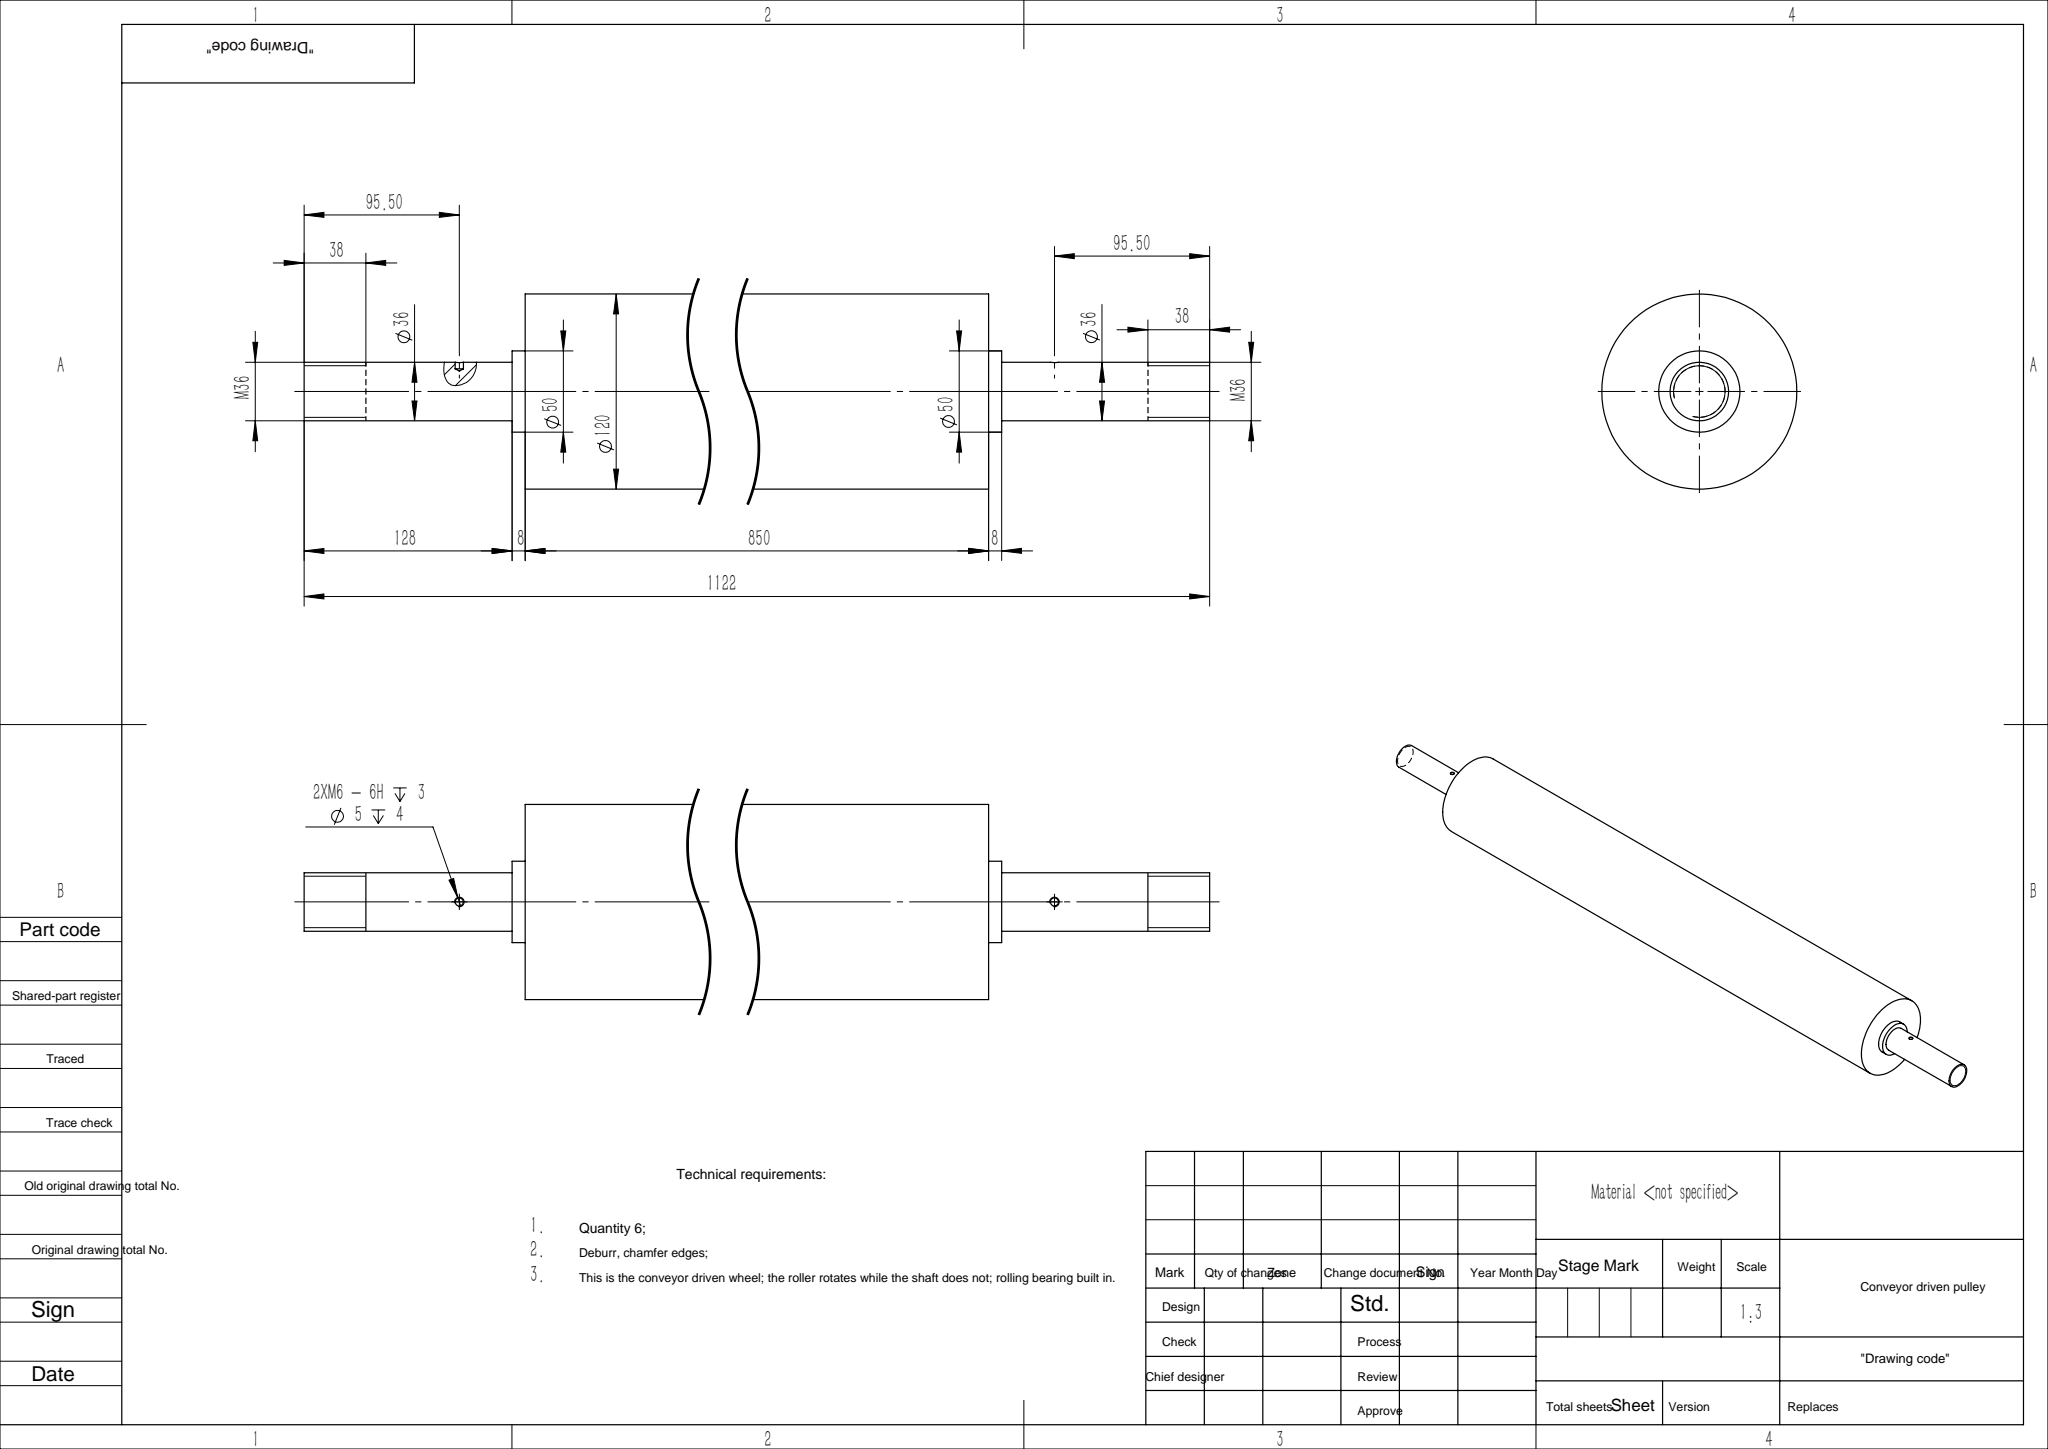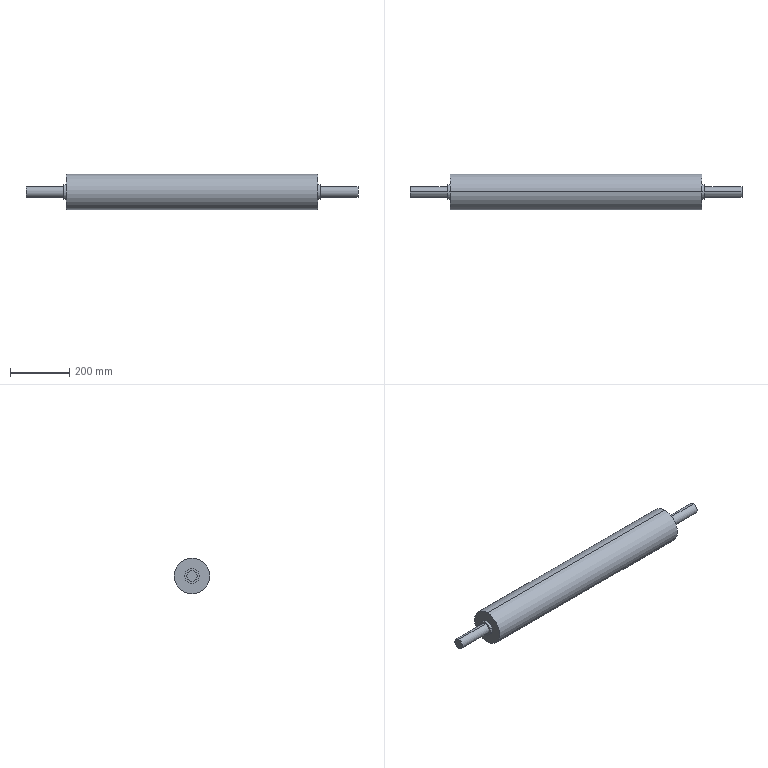Part | SolidWorks | features 3DProfileFeature 1, HoleWzd 1, MirrorPattern 1, Revolution 1 | 1 solid | 24 faces | box 1122 x 120 x 120 mm | volume 9905091 mm3 | cylinder 14 | plane 6 | cone 4 | commonest cylinder face diameters 5 x4 36 x4 50 x4 120 x2
STEP:
#1=CARTESIAN_POINT('',(-465.5,12.557,0.));
#2=VERTEX_POINT('',#1);
#3=CARTESIAN_POINT('',(-465.5,14.,2.5));
#4=VERTEX_POINT('',#3);
#5=CARTESIAN_POINT('',(-465.5,14.,2.5));
#6=DIRECTION('',(0.,0.5,0.866));
#7=VECTOR('',#6,1000.);
#8=LINE('',#5,#7);
#9=EDGE_CURVE('',#2,#4,#8,.T.);
#10=ORIENTED_EDGE('',*,*,#9,.F.);
#11=CARTESIAN_POINT('',(-465.5,14.,-2.5));
#12=VERTEX_POINT('',#11);
#13=CARTESIAN_POINT('',(-465.5,14.,-2.5));
#14=DIRECTION('',(0.,0.5,-0.866));
#15=VECTOR('',#14,1000.);
#16=LINE('',#13,#15);
#17=EDGE_CURVE('',#2,#12,#16,.T.);
#18=ORIENTED_EDGE('',*,*,#17,.T.);
#19=CARTESIAN_POINT('',(-465.5,14.,0.));
#20=DIRECTION('',(0.,1.,0.));
#21=DIRECTION('',(0.,0.,1.));
#22=AXIS2_PLACEMENT_3D('',#19,#20,#21);
#23=CIRCLE('',#22,2.5);
#24=EDGE_CURVE('',#12,#4,#23,.T.);
#25=ORIENTED_EDGE('',*,*,#24,.T.);
#26=EDGE_LOOP('',(#10,#18,#25));
#27=FACE_OUTER_BOUND('',#26,.T.);
#28=CARTESIAN_POINT('',(-465.5,14.,0.));
#29=DIRECTION('',(0.,1.,0.));
#30=DIRECTION('',(0.,0.,1.));
#31=AXIS2_PLACEMENT_3D('',#28,#29,#30);
#32=CONICAL_SURFACE('',#31,2.5,1.047);
#33=ADVANCED_FACE('',(#27),#32,.F.);
#34=ORIENTED_EDGE('',*,*,#24,.F.);
#35=CARTESIAN_POINT('',(-465.5,17.826,-2.5));
#36=VERTEX_POINT('',#35);
#37=CARTESIAN_POINT('',(-465.5,18.,-2.5));
#38=DIRECTION('',(0.,1.,0.));
#39=VECTOR('',#38,1000.);
#40=LINE('',#37,#39);
#41=EDGE_CURVE('',#12,#36,#40,.T.);
#42=ORIENTED_EDGE('',*,*,#41,.T.);
#43=CARTESIAN_POINT('',(-465.5,17.826,2.5));
#44=VERTEX_POINT('',#43);
#45=CARTESIAN_POINT('',(-465.5,17.826,2.5));
#46=CARTESIAN_POINT('',(-465.665,17.826,2.5));
#47=CARTESIAN_POINT('',(-465.828,17.828,2.484));
#48=CARTESIAN_POINT('',(-466.148,17.837,2.42));
#49=CARTESIAN_POINT('',(-466.307,17.843,2.372));
#50=CARTESIAN_POINT('',(-466.609,17.859,2.246));
#51=CARTESIAN_POINT('',(-466.753,17.869,2.17));
#52=CARTESIAN_POINT('',(-467.025,17.89,1.988));
#53=CARTESIAN_POINT('',(-467.153,17.902,1.883));
#54=CARTESIAN_POINT('',(-467.383,17.924,1.652));
#55=CARTESIAN_POINT('',(-467.487,17.936,1.526));
#56=CARTESIAN_POINT('',(-467.669,17.957,1.253));
#57=CARTESIAN_POINT('',(-467.747,17.966,1.108));
#58=CARTESIAN_POINT('',(-467.872,17.983,0.8072));
#59=CARTESIAN_POINT('',(-467.92,17.989,0.6494));
#60=CARTESIAN_POINT('',(-467.984,17.998,0.3266));
#61=CARTESIAN_POINT('',(-468.,18.,0.1642));
#62=CARTESIAN_POINT('',(-468.,18.,-0.1624));
#63=CARTESIAN_POINT('',(-467.984,17.998,-0.3282));
#64=CARTESIAN_POINT('',(-467.92,17.989,-0.649));
#65=CARTESIAN_POINT('',(-467.873,17.983,-0.805));
#66=CARTESIAN_POINT('',(-467.747,17.967,-1.108));
#67=CARTESIAN_POINT('',(-467.669,17.957,-1.254));
#68=CARTESIAN_POINT('',(-467.488,17.936,-1.525));
#69=CARTESIAN_POINT('',(-467.384,17.924,-1.651));
#70=CARTESIAN_POINT('',(-467.151,17.901,-1.884));
#71=CARTESIAN_POINT('',(-467.025,17.89,-1.987));
#72=CARTESIAN_POINT('',(-466.755,17.869,-2.168));
#73=CARTESIAN_POINT('',(-466.608,17.859,-2.247));
#74=CARTESIAN_POINT('',(-466.306,17.843,-2.372));
#75=CARTESIAN_POINT('',(-466.15,17.837,-2.42));
#76=CARTESIAN_POINT('',(-465.829,17.828,-2.484));
#77=CARTESIAN_POINT('',(-465.663,17.826,-2.5));
#78=CARTESIAN_POINT('',(-465.5,17.826,-2.5));
#79=B_SPLINE_CURVE_WITH_KNOTS('',3,(#45,#46,#47,#48,#49,#50,#51,#52,#53,#54,#55,#56,#57,#58,#59,#60,#61,#62,#63,#64,#65,#66,#67,#68,#69,#70,#71,#72,#73,#74,#75,#76,#77,#78),.UNSPECIFIED.,.F.,.F.,(4,2,2,2,2,2,2,2,2,2,2,2,2,2,2,2,4),(0.,0.0004891,0.0009782,0.001467,0.001956,0.002445,0.002935,0.003424,0.003913,0.004402,0.004891,0.00538,0.005869,0.006358,0.006847,0.007336,0.007826),.UNSPECIFIED.);
#80=EDGE_CURVE('',#44,#36,#79,.T.);
#81=ORIENTED_EDGE('',*,*,#80,.F.);
#82=CARTESIAN_POINT('',(-465.5,18.,2.5));
#83=DIRECTION('',(0.,1.,0.));
#84=VECTOR('',#83,1000.);
#85=LINE('',#82,#84);
#86=EDGE_CURVE('',#4,#44,#85,.T.);
#87=ORIENTED_EDGE('',*,*,#86,.F.);
#88=EDGE_LOOP('',(#34,#42,#81,#87));
#89=FACE_OUTER_BOUND('',#88,.T.);
#90=CARTESIAN_POINT('',(-465.5,18.,0.));
#91=DIRECTION('',(0.,1.,0.));
#92=DIRECTION('',(0.,0.,1.));
#93=AXIS2_PLACEMENT_3D('',#90,#91,#92);
#94=CYLINDRICAL_SURFACE('',#93,2.5);
#95=ADVANCED_FACE('',(#89),#94,.F.);
#96=CARTESIAN_POINT('',(465.5,12.557,0.));
#97=VERTEX_POINT('',#96);
#98=CARTESIAN_POINT('',(465.5,14.,2.5));
#99=VERTEX_POINT('',#98);
#100=CARTESIAN_POINT('',(465.5,14.,2.5));
#101=DIRECTION('',(0.,0.5,0.866));
#102=VECTOR('',#101,1000.);
#103=LINE('',#100,#102);
#104=EDGE_CURVE('',#97,#99,#103,.T.);
#105=ORIENTED_EDGE('',*,*,#104,.F.);
#106=CARTESIAN_POINT('',(465.5,14.,-2.5));
#107=VERTEX_POINT('',#106);
#108=CARTESIAN_POINT('',(465.5,14.,-2.5));
#109=DIRECTION('',(0.,0.5,-0.866));
#110=VECTOR('',#109,1000.);
#111=LINE('',#108,#110);
#112=EDGE_CURVE('',#97,#107,#111,.T.);
#113=ORIENTED_EDGE('',*,*,#112,.T.);
#114=CARTESIAN_POINT('',(465.5,14.,0.));
#115=DIRECTION('',(0.,1.,0.));
#116=DIRECTION('',(0.,0.,1.));
#117=AXIS2_PLACEMENT_3D('',#114,#115,#116);
#118=CIRCLE('',#117,2.5);
#119=EDGE_CURVE('',#107,#99,#118,.T.);
#120=ORIENTED_EDGE('',*,*,#119,.T.);
#121=EDGE_LOOP('',(#105,#113,#120));
#122=FACE_OUTER_BOUND('',#121,.T.);
#123=CARTESIAN_POINT('',(465.5,14.,0.));
#124=DIRECTION('',(0.,1.,0.));
#125=DIRECTION('',(0.,0.,1.));
#126=AXIS2_PLACEMENT_3D('',#123,#124,#125);
#127=CONICAL_SURFACE('',#126,2.5,1.047);
#128=ADVANCED_FACE('',(#122),#127,.F.);
#129=ORIENTED_EDGE('',*,*,#119,.F.);
#130=CARTESIAN_POINT('',(465.5,17.826,-2.5));
#131=VERTEX_POINT('',#130);
#132=CARTESIAN_POINT('',(465.5,18.,-2.5));
#133=DIRECTION('',(0.,1.,0.));
#134=VECTOR('',#133,1000.);
#135=LINE('',#132,#134);
#136=EDGE_CURVE('',#107,#131,#135,.T.);
#137=ORIENTED_EDGE('',*,*,#136,.T.);
#138=CARTESIAN_POINT('',(465.5,17.826,2.5));
#139=VERTEX_POINT('',#138);
#140=CARTESIAN_POINT('',(465.5,17.826,2.5));
#141=CARTESIAN_POINT('',(465.335,17.826,2.5));
#142=CARTESIAN_POINT('',(465.172,17.828,2.484));
#143=CARTESIAN_POINT('',(464.852,17.837,2.42));
#144=CARTESIAN_POINT('',(464.693,17.843,2.372));
#145=CARTESIAN_POINT('',(464.391,17.859,2.246));
#146=CARTESIAN_POINT('',(464.247,17.869,2.17));
#147=CARTESIAN_POINT('',(463.975,17.89,1.988));
#148=CARTESIAN_POINT('',(463.847,17.902,1.883));
#149=CARTESIAN_POINT('',(463.617,17.924,1.652));
#150=CARTESIAN_POINT('',(463.513,17.936,1.526));
#151=CARTESIAN_POINT('',(463.331,17.957,1.253));
#152=CARTESIAN_POINT('',(463.253,17.966,1.108));
#153=CARTESIAN_POINT('',(463.128,17.983,0.8072));
#154=CARTESIAN_POINT('',(463.08,17.989,0.6494));
#155=CARTESIAN_POINT('',(463.016,17.998,0.3266));
#156=CARTESIAN_POINT('',(463.,18.,0.1642));
#157=CARTESIAN_POINT('',(463.,18.,-0.1624));
#158=CARTESIAN_POINT('',(463.016,17.998,-0.3282));
#159=CARTESIAN_POINT('',(463.08,17.989,-0.649));
#160=CARTESIAN_POINT('',(463.127,17.983,-0.805));
#161=CARTESIAN_POINT('',(463.253,17.967,-1.108));
#162=CARTESIAN_POINT('',(463.331,17.957,-1.254));
#163=CARTESIAN_POINT('',(463.512,17.936,-1.525));
#164=CARTESIAN_POINT('',(463.616,17.924,-1.651));
#165=CARTESIAN_POINT('',(463.849,17.901,-1.884));
#166=CARTESIAN_POINT('',(463.975,17.89,-1.987));
#167=CARTESIAN_POINT('',(464.245,17.869,-2.168));
#168=CARTESIAN_POINT('',(464.392,17.859,-2.247));
#169=CARTESIAN_POINT('',(464.694,17.843,-2.372));
#170=CARTESIAN_POINT('',(464.85,17.837,-2.42));
#171=CARTESIAN_POINT('',(465.171,17.828,-2.484));
#172=CARTESIAN_POINT('',(465.337,17.826,-2.5));
#173=CARTESIAN_POINT('',(465.5,17.826,-2.5));
#174=B_SPLINE_CURVE_WITH_KNOTS('',3,(#140,#141,#142,#143,#144,#145,#146,#147,#148,#149,#150,#151,#152,#153,#154,#155,#156,#157,#158,#159,#160,#161,#162,#163,#164,#165,#166,#167,#168,#169,#170,#171,#172,#173),.UNSPECIFIED.,.F.,.F.,(4,2,2,2,2,2,2,2,2,2,2,2,2,2,2,2,4),(0.,0.0004891,0.0009782,0.001467,0.001956,0.002445,0.002935,0.003424,0.003913,0.004402,0.004891,0.00538,0.005869,0.006358,0.006847,0.007336,0.007826),.UNSPECIFIED.);
#175=EDGE_CURVE('',#139,#131,#174,.T.);
#176=ORIENTED_EDGE('',*,*,#175,.F.);
#177=CARTESIAN_POINT('',(465.5,18.,2.5));
#178=DIRECTION('',(0.,1.,0.));
#179=VECTOR('',#178,1000.);
#180=LINE('',#177,#179);
#181=EDGE_CURVE('',#99,#139,#180,.T.);
#182=ORIENTED_EDGE('',*,*,#181,.F.);
#183=EDGE_LOOP('',(#129,#137,#176,#182));
#184=FACE_OUTER_BOUND('',#183,.T.);
#185=CARTESIAN_POINT('',(465.5,18.,0.));
#186=DIRECTION('',(0.,1.,0.));
#187=DIRECTION('',(0.,0.,1.));
#188=AXIS2_PLACEMENT_3D('',#185,#186,#187);
#189=CYLINDRICAL_SURFACE('',#188,2.5);
#190=ADVANCED_FACE('',(#184),#189,.F.);
#191=CARTESIAN_POINT('',(425.,0.,60.));
#192=VERTEX_POINT('',#191);
#193=CARTESIAN_POINT('',(425.,0.,-60.));
#194=VERTEX_POINT('',#193);
#195=CARTESIAN_POINT('',(425.,0.,0.));
#196=DIRECTION('',(-1.,0.,0.));
#197=DIRECTION('',(0.,0.,1.));
#198=AXIS2_PLACEMENT_3D('',#195,#196,#197);
#199=CIRCLE('',#198,60.);
#200=EDGE_CURVE('',#192,#194,#199,.T.);
#201=ORIENTED_EDGE('',*,*,#200,.T.);
#202=CARTESIAN_POINT('',(-425.,0.,-60.));
#203=VERTEX_POINT('',#202);
#204=CARTESIAN_POINT('',(0.,0.,-60.));
#205=DIRECTION('',(-1.,0.,0.));
#206=VECTOR('',#205,1000.);
#207=LINE('',#204,#206);
#208=EDGE_CURVE('',#194,#203,#207,.T.);
#209=ORIENTED_EDGE('',*,*,#208,.T.);
#210=CARTESIAN_POINT('',(-425.,0.,60.));
#211=VERTEX_POINT('',#210);
#212=CARTESIAN_POINT('',(-425.,0.,0.));
#213=DIRECTION('',(-1.,0.,0.));
#214=DIRECTION('',(0.,0.,1.));
#215=AXIS2_PLACEMENT_3D('',#212,#213,#214);
#216=CIRCLE('',#215,60.);
#217=EDGE_CURVE('',#211,#203,#216,.T.);
#218=ORIENTED_EDGE('',*,*,#217,.F.);
#219=CARTESIAN_POINT('',(0.,0.,60.));
#220=DIRECTION('',(-1.,0.,0.));
#221=VECTOR('',#220,1000.);
#222=LINE('',#219,#221);
#223=EDGE_CURVE('',#192,#211,#222,.T.);
#224=ORIENTED_EDGE('',*,*,#223,.F.);
#225=EDGE_LOOP('',(#201,#209,#218,#224));
#226=FACE_OUTER_BOUND('',#225,.T.);
#227=CARTESIAN_POINT('',(0.,0.,0.));
#228=DIRECTION('',(-1.,0.,0.));
#229=DIRECTION('',(0.,0.,1.));
#230=AXIS2_PLACEMENT_3D('',#227,#228,#229);
#231=CYLINDRICAL_SURFACE('',#230,60.);
#232=ADVANCED_FACE('',(#226),#231,.T.);
#233=CARTESIAN_POINT('',(-425.,0.,25.));
#234=VERTEX_POINT('',#233);
#235=CARTESIAN_POINT('',(-425.,0.,-25.));
#236=VERTEX_POINT('',#235);
#237=CARTESIAN_POINT('',(-425.,0.,0.));
#238=DIRECTION('',(-1.,0.,0.));
#239=DIRECTION('',(0.,0.,1.));
#240=AXIS2_PLACEMENT_3D('',#237,#238,#239);
#241=CIRCLE('',#240,25.);
#242=EDGE_CURVE('',#234,#236,#241,.T.);
#243=ORIENTED_EDGE('',*,*,#242,.T.);
#244=CARTESIAN_POINT('',(-433.,0.,-25.));
#245=VERTEX_POINT('',#244);
#246=CARTESIAN_POINT('',(0.,0.,-25.));
#247=DIRECTION('',(-1.,0.,0.));
#248=VECTOR('',#247,1000.);
#249=LINE('',#246,#248);
#250=EDGE_CURVE('',#236,#245,#249,.T.);
#251=ORIENTED_EDGE('',*,*,#250,.T.);
#252=CARTESIAN_POINT('',(-433.,0.,25.));
#253=VERTEX_POINT('',#252);
#254=CARTESIAN_POINT('',(-433.,0.,0.));
#255=DIRECTION('',(-1.,0.,0.));
#256=DIRECTION('',(0.,0.,1.));
#257=AXIS2_PLACEMENT_3D('',#254,#255,#256);
#258=CIRCLE('',#257,25.);
#259=EDGE_CURVE('',#253,#245,#258,.T.);
#260=ORIENTED_EDGE('',*,*,#259,.F.);
#261=CARTESIAN_POINT('',(0.,0.,25.));
#262=DIRECTION('',(-1.,0.,0.));
#263=VECTOR('',#262,1000.);
#264=LINE('',#261,#263);
#265=EDGE_CURVE('',#234,#253,#264,.T.);
#266=ORIENTED_EDGE('',*,*,#265,.F.);
#267=EDGE_LOOP('',(#243,#251,#260,#266));
#268=FACE_OUTER_BOUND('',#267,.T.);
#269=CARTESIAN_POINT('',(0.,0.,0.));
#270=DIRECTION('',(-1.,0.,0.));
#271=DIRECTION('',(0.,0.,1.));
#272=AXIS2_PLACEMENT_3D('',#269,#270,#271);
#273=CYLINDRICAL_SURFACE('',#272,25.);
#274=ADVANCED_FACE('',(#268),#273,.T.);
#275=ORIENTED_EDGE('',*,*,#80,.T.);
#276=CARTESIAN_POINT('',(-465.5,17.826,-2.5));
#277=CARTESIAN_POINT('',(-465.337,17.826,-2.5));
#278=CARTESIAN_POINT('',(-465.174,17.828,-2.484));
#279=CARTESIAN_POINT('',(-464.851,17.837,-2.42));
#280=CARTESIAN_POINT('',(-464.694,17.843,-2.372));
#281=CARTESIAN_POINT('',(-464.393,17.859,-2.247));
#282=CARTESIAN_POINT('',(-464.247,17.869,-2.17));
#283=CARTESIAN_POINT('',(-463.974,17.89,-1.987));
#284=CARTESIAN_POINT('',(-463.849,17.901,-1.884));
#285=CARTESIAN_POINT('',(-463.618,17.924,-1.654));
#286=CARTESIAN_POINT('',(-463.513,17.936,-1.525));
#287=CARTESIAN_POINT('',(-463.331,17.957,-1.254));
#288=CARTESIAN_POINT('',(-463.254,17.966,-1.111));
#289=CARTESIAN_POINT('',(-463.129,17.982,-0.808));
#290=CARTESIAN_POINT('',(-463.08,17.989,-0.6493));
#291=CARTESIAN_POINT('',(-463.016,17.998,-0.3297));
#292=CARTESIAN_POINT('',(-463.,18.,-0.167));
#293=CARTESIAN_POINT('',(-463.,18.,0.1636));
#294=CARTESIAN_POINT('',(-463.016,17.998,0.3261));
#295=CARTESIAN_POINT('',(-463.079,17.989,0.6459));
#296=CARTESIAN_POINT('',(-463.127,17.983,0.8049));
#297=CARTESIAN_POINT('',(-463.253,17.967,1.108));
#298=CARTESIAN_POINT('',(-463.329,17.957,1.251));
#299=CARTESIAN_POINT('',(-463.511,17.936,1.523));
#300=CARTESIAN_POINT('',(-463.616,17.924,1.651));
#301=CARTESIAN_POINT('',(-463.961,17.89,1.997));
#302=CARTESIAN_POINT('',(-464.24,17.868,2.183));
#303=CARTESIAN_POINT('',(-464.841,17.835,2.433));
#304=CARTESIAN_POINT('',(-465.169,17.826,2.5));
#305=CARTESIAN_POINT('',(-465.5,17.826,2.5));
#306=B_SPLINE_CURVE_WITH_KNOTS('',3,(#276,#277,#278,#279,#280,#281,#282,#283,#284,#285,#286,#287,#288,#289,#290,#291,#292,#293,#294,#295,#296,#297,#298,#299,#300,#301,#302,#303,#304,#305),.UNSPECIFIED.,.F.,.F.,(4,2,2,2,2,2,2,2,2,2,2,2,2,2,4),(0.007826,0.008315,0.008804,0.009293,0.009782,0.01027,0.01076,0.01125,0.01174,0.01223,0.01272,0.0132,0.01369,0.01467,0.01565),.UNSPECIFIED.);
#307=EDGE_CURVE('',#36,#44,#306,.T.);
#308=ORIENTED_EDGE('',*,*,#307,.T.);
#309=EDGE_LOOP('',(#275,#308));
#310=FACE_BOUND('',#309,.T.);
#311=CARTESIAN_POINT('',(-433.,0.,18.));
#312=VERTEX_POINT('',#311);
#313=CARTESIAN_POINT('',(-433.,0.,-18.));
#314=VERTEX_POINT('',#313);
#315=CARTESIAN_POINT('',(-433.,0.,0.));
#316=DIRECTION('',(-1.,0.,0.));
#317=DIRECTION('',(0.,0.,1.));
#318=AXIS2_PLACEMENT_3D('',#315,#316,#317);
#319=CIRCLE('',#318,18.);
#320=EDGE_CURVE('',#312,#314,#319,.T.);
#321=ORIENTED_EDGE('',*,*,#320,.T.);
#322=CARTESIAN_POINT('',(-561.,0.,-18.));
#323=VERTEX_POINT('',#322);
#324=CARTESIAN_POINT('',(0.,0.,-18.));
#325=DIRECTION('',(-1.,0.,0.));
#326=VECTOR('',#325,1000.);
#327=LINE('',#324,#326);
#328=EDGE_CURVE('',#314,#323,#327,.T.);
#329=ORIENTED_EDGE('',*,*,#328,.T.);
#330=CARTESIAN_POINT('',(-561.,0.,18.));
#331=VERTEX_POINT('',#330);
#332=CARTESIAN_POINT('',(-561.,0.,0.));
#333=DIRECTION('',(-1.,0.,0.));
#334=DIRECTION('',(0.,0.,1.));
#335=AXIS2_PLACEMENT_3D('',#332,#333,#334);
#336=CIRCLE('',#335,18.);
#337=EDGE_CURVE('',#331,#323,#336,.T.);
#338=ORIENTED_EDGE('',*,*,#337,.F.);
#339=CARTESIAN_POINT('',(0.,0.,18.));
#340=DIRECTION('',(-1.,0.,0.));
#341=VECTOR('',#340,1000.);
#342=LINE('',#339,#341);
#343=EDGE_CURVE('',#312,#331,#342,.T.);
#344=ORIENTED_EDGE('',*,*,#343,.F.);
#345=EDGE_LOOP('',(#321,#329,#338,#344));
#346=FACE_OUTER_BOUND('',#345,.T.);
#347=CARTESIAN_POINT('',(0.,0.,0.));
#348=DIRECTION('',(-1.,0.,0.));
#349=DIRECTION('',(0.,0.,1.));
#350=AXIS2_PLACEMENT_3D('',#347,#348,#349);
#351=CYLINDRICAL_SURFACE('',#350,18.);
#352=ADVANCED_FACE('',(#310,#346),#351,.T.);
#353=ORIENTED_EDGE('',*,*,#175,.T.);
#354=CARTESIAN_POINT('',(465.5,17.826,-2.5));
#355=CARTESIAN_POINT('',(465.663,17.826,-2.5));
#356=CARTESIAN_POINT('',(465.826,17.828,-2.484));
#357=CARTESIAN_POINT('',(466.149,17.837,-2.42));
#358=CARTESIAN_POINT('',(466.306,17.843,-2.372));
#359=CARTESIAN_POINT('',(466.607,17.859,-2.247));
#360=CARTESIAN_POINT('',(466.753,17.869,-2.17));
#361=CARTESIAN_POINT('',(467.026,17.89,-1.987));
#362=CARTESIAN_POINT('',(467.151,17.901,-1.884));
#363=CARTESIAN_POINT('',(467.382,17.924,-1.654));
#364=CARTESIAN_POINT('',(467.487,17.936,-1.525));
#365=CARTESIAN_POINT('',(467.669,17.957,-1.254));
#366=CARTESIAN_POINT('',(467.746,17.966,-1.111));
#367=CARTESIAN_POINT('',(467.871,17.982,-0.808));
#368=CARTESIAN_POINT('',(467.92,17.989,-0.6493));
#369=CARTESIAN_POINT('',(467.984,17.998,-0.3297));
#370=CARTESIAN_POINT('',(468.,18.,-0.167));
#371=CARTESIAN_POINT('',(468.,18.,0.1636));
#372=CARTESIAN_POINT('',(467.984,17.998,0.3261));
#373=CARTESIAN_POINT('',(467.921,17.989,0.6459));
#374=CARTESIAN_POINT('',(467.873,17.983,0.8049));
#375=CARTESIAN_POINT('',(467.747,17.967,1.108));
#376=CARTESIAN_POINT('',(467.671,17.957,1.251));
#377=CARTESIAN_POINT('',(467.489,17.936,1.523));
#378=CARTESIAN_POINT('',(467.384,17.924,1.651));
#379=CARTESIAN_POINT('',(467.039,17.89,1.997));
#380=CARTESIAN_POINT('',(466.76,17.868,2.183));
#381=CARTESIAN_POINT('',(466.159,17.835,2.433));
#382=CARTESIAN_POINT('',(465.831,17.826,2.5));
#383=CARTESIAN_POINT('',(465.5,17.826,2.5));
#384=B_SPLINE_CURVE_WITH_KNOTS('',3,(#354,#355,#356,#357,#358,#359,#360,#361,#362,#363,#364,#365,#366,#367,#368,#369,#370,#371,#372,#373,#374,#375,#376,#377,#378,#379,#380,#381,#382,#383),.UNSPECIFIED.,.F.,.F.,(4,2,2,2,2,2,2,2,2,2,2,2,2,2,4),(0.007826,0.008315,0.008804,0.009293,0.009782,0.01027,0.01076,0.01125,0.01174,0.01223,0.01272,0.0132,0.01369,0.01467,0.01565),.UNSPECIFIED.);
#385=EDGE_CURVE('',#131,#139,#384,.T.);
#386=ORIENTED_EDGE('',*,*,#385,.T.);
#387=EDGE_LOOP('',(#353,#386));
#388=FACE_BOUND('',#387,.T.);
#389=CARTESIAN_POINT('',(561.,0.,18.));
#390=VERTEX_POINT('',#389);
#391=CARTESIAN_POINT('',(561.,0.,-18.));
#392=VERTEX_POINT('',#391);
#393=CARTESIAN_POINT('',(561.,0.,0.));
#394=DIRECTION('',(-1.,0.,0.));
#395=DIRECTION('',(0.,0.,1.));
#396=AXIS2_PLACEMENT_3D('',#393,#394,#395);
#397=CIRCLE('',#396,18.);
#398=EDGE_CURVE('',#390,#392,#397,.T.);
#399=ORIENTED_EDGE('',*,*,#398,.T.);
#400=CARTESIAN_POINT('',(433.,0.,-18.));
#401=VERTEX_POINT('',#400);
#402=CARTESIAN_POINT('',(0.,0.,-18.));
#403=DIRECTION('',(-1.,0.,0.));
#404=VECTOR('',#403,1000.);
#405=LINE('',#402,#404);
#406=EDGE_CURVE('',#392,#401,#405,.T.);
#407=ORIENTED_EDGE('',*,*,#406,.T.);
#408=CARTESIAN_POINT('',(433.,0.,18.));
#409=VERTEX_POINT('',#408);
#410=CARTESIAN_POINT('',(433.,0.,0.));
#411=DIRECTION('',(-1.,0.,0.));
#412=DIRECTION('',(0.,0.,1.));
#413=AXIS2_PLACEMENT_3D('',#410,#411,#412);
#414=CIRCLE('',#413,18.);
#415=EDGE_CURVE('',#409,#401,#414,.T.);
#416=ORIENTED_EDGE('',*,*,#415,.F.);
#417=CARTESIAN_POINT('',(0.,0.,18.));
#418=DIRECTION('',(-1.,0.,0.));
#419=VECTOR('',#418,1000.);
#420=LINE('',#417,#419);
#421=EDGE_CURVE('',#390,#409,#420,.T.);
#422=ORIENTED_EDGE('',*,*,#421,.F.);
#423=EDGE_LOOP('',(#399,#407,#416,#422));
#424=FACE_OUTER_BOUND('',#423,.T.);
#425=CARTESIAN_POINT('',(0.,0.,0.));
#426=DIRECTION('',(-1.,0.,0.));
#427=DIRECTION('',(0.,0.,1.));
#428=AXIS2_PLACEMENT_3D('',#425,#426,#427);
#429=CYLINDRICAL_SURFACE('',#428,18.);
#430=ADVANCED_FACE('',(#388,#424),#429,.T.);
#431=CARTESIAN_POINT('',(433.,0.,25.));
#432=VERTEX_POINT('',#431);
#433=CARTESIAN_POINT('',(433.,0.,-25.));
#434=VERTEX_POINT('',#433);
#435=CARTESIAN_POINT('',(433.,0.,0.));
#436=DIRECTION('',(-1.,0.,0.));
#437=DIRECTION('',(0.,0.,1.));
#438=AXIS2_PLACEMENT_3D('',#435,#436,#437);
#439=CIRCLE('',#438,25.);
#440=EDGE_CURVE('',#432,#434,#439,.T.);
#441=ORIENTED_EDGE('',*,*,#440,.T.);
#442=CARTESIAN_POINT('',(425.,0.,-25.));
#443=VERTEX_POINT('',#442);
#444=CARTESIAN_POINT('',(0.,0.,-25.));
#445=DIRECTION('',(-1.,0.,0.));
#446=VECTOR('',#445,1000.);
#447=LINE('',#444,#446);
#448=EDGE_CURVE('',#434,#443,#447,.T.);
#449=ORIENTED_EDGE('',*,*,#448,.T.);
#450=CARTESIAN_POINT('',(425.,0.,25.));
#451=VERTEX_POINT('',#450);
#452=CARTESIAN_POINT('',(425.,0.,0.));
#453=DIRECTION('',(-1.,0.,0.));
#454=DIRECTION('',(0.,0.,1.));
#455=AXIS2_PLACEMENT_3D('',#452,#453,#454);
#456=CIRCLE('',#455,25.);
#457=EDGE_CURVE('',#451,#443,#456,.T.);
#458=ORIENTED_EDGE('',*,*,#457,.F.);
#459=CARTESIAN_POINT('',(0.,0.,25.));
#460=DIRECTION('',(-1.,0.,0.));
#461=VECTOR('',#460,1000.);
#462=LINE('',#459,#461);
#463=EDGE_CURVE('',#432,#451,#462,.T.);
#464=ORIENTED_EDGE('',*,*,#463,.F.);
#465=EDGE_LOOP('',(#441,#449,#458,#464));
#466=FACE_OUTER_BOUND('',#465,.T.);
#467=CARTESIAN_POINT('',(0.,0.,0.));
#468=DIRECTION('',(-1.,0.,0.));
#469=DIRECTION('',(0.,0.,1.));
#470=AXIS2_PLACEMENT_3D('',#467,#468,#469);
#471=CYLINDRICAL_SURFACE('',#470,25.);
#472=ADVANCED_FACE('',(#466),#471,.T.);
#473=ORIENTED_EDGE('',*,*,#448,.F.);
#474=CARTESIAN_POINT('',(433.,0.,0.));
#475=DIRECTION('',(-1.,0.,0.));
#476=DIRECTION('',(0.,0.,1.));
#477=AXIS2_PLACEMENT_3D('',#474,#475,#476);
#478=CIRCLE('',#477,25.);
#479=EDGE_CURVE('',#434,#432,#478,.T.);
#480=ORIENTED_EDGE('',*,*,#479,.T.);
#481=ORIENTED_EDGE('',*,*,#463,.T.);
#482=CARTESIAN_POINT('',(425.,0.,0.));
#483=DIRECTION('',(-1.,0.,0.));
#484=DIRECTION('',(0.,0.,1.));
#485=AXIS2_PLACEMENT_3D('',#482,#483,#484);
#486=CIRCLE('',#485,25.);
#487=EDGE_CURVE('',#443,#451,#486,.T.);
#488=ORIENTED_EDGE('',*,*,#487,.F.);
#489=EDGE_LOOP('',(#473,#480,#481,#488));
#490=FACE_OUTER_BOUND('',#489,.T.);
#491=CARTESIAN_POINT('',(0.,0.,0.));
#492=DIRECTION('',(-1.,0.,0.));
#493=DIRECTION('',(0.,0.,1.));
#494=AXIS2_PLACEMENT_3D('',#491,#492,#493);
#495=CYLINDRICAL_SURFACE('',#494,25.);
#496=ADVANCED_FACE('',(#490),#495,.T.);
#497=ORIENTED_EDGE('',*,*,#440,.F.);
#498=ORIENTED_EDGE('',*,*,#479,.F.);
#499=EDGE_LOOP('',(#497,#498));
#500=FACE_OUTER_BOUND('',#499,.T.);
#501=ORIENTED_EDGE('',*,*,#415,.T.);
#502=CARTESIAN_POINT('',(433.,0.,0.));
#503=DIRECTION('',(-1.,0.,0.));
#504=DIRECTION('',(0.,0.,1.));
#505=AXIS2_PLACEMENT_3D('',#502,#503,#504);
#506=CIRCLE('',#505,18.);
#507=EDGE_CURVE('',#401,#409,#506,.T.);
#508=ORIENTED_EDGE('',*,*,#507,.T.);
#509=EDGE_LOOP('',(#501,#508));
#510=FACE_BOUND('',#509,.T.);
#511=CARTESIAN_POINT('',(433.,25.,0.));
#512=DIRECTION('',(-1.,0.,0.));
#513=DIRECTION('',(0.,0.,1.));
#514=AXIS2_PLACEMENT_3D('',#511,#512,#513);
#515=PLANE('',#514);
#516=ADVANCED_FACE('',(#500,#510),#515,.F.);
#517=ORIENTED_EDGE('',*,*,#406,.F.);
#518=CARTESIAN_POINT('',(561.,0.,0.));
#519=DIRECTION('',(-1.,0.,0.));
#520=DIRECTION('',(0.,0.,1.));
#521=AXIS2_PLACEMENT_3D('',#518,#519,#520);
#522=CIRCLE('',#521,18.);
#523=EDGE_CURVE('',#392,#390,#522,.T.);
#524=ORIENTED_EDGE('',*,*,#523,.T.);
#525=ORIENTED_EDGE('',*,*,#421,.T.);
#526=ORIENTED_EDGE('',*,*,#507,.F.);
#527=EDGE_LOOP('',(#517,#524,#525,#526));
#528=FACE_OUTER_BOUND('',#527,.T.);
#529=CARTESIAN_POINT('',(0.,0.,0.));
#530=DIRECTION('',(-1.,0.,0.));
#531=DIRECTION('',(0.,0.,1.));
#532=AXIS2_PLACEMENT_3D('',#529,#530,#531);
#533=CYLINDRICAL_SURFACE('',#532,18.);
#534=ADVANCED_FACE('',(#528),#533,.T.);
#535=ORIENTED_EDGE('',*,*,#398,.F.);
#536=ORIENTED_EDGE('',*,*,#523,.F.);
#537=EDGE_LOOP('',(#535,#536));
#538=FACE_OUTER_BOUND('',#537,.T.);
#539=CARTESIAN_POINT('',(561.,18.,0.));
#540=DIRECTION('',(-1.,0.,0.));
#541=DIRECTION('',(0.,0.,1.));
#542=AXIS2_PLACEMENT_3D('',#539,#540,#541);
#543=PLANE('',#542);
#544=ADVANCED_FACE('',(#538),#543,.F.);
#545=ORIENTED_EDGE('',*,*,#337,.T.);
#546=CARTESIAN_POINT('',(-561.,0.,0.));
#547=DIRECTION('',(-1.,0.,0.));
#548=DIRECTION('',(0.,0.,1.));
#549=AXIS2_PLACEMENT_3D('',#546,#547,#548);
#550=CIRCLE('',#549,18.);
#551=EDGE_CURVE('',#323,#331,#550,.T.);
#552=ORIENTED_EDGE('',*,*,#551,.T.);
#553=EDGE_LOOP('',(#545,#552));
#554=FACE_OUTER_BOUND('',#553,.T.);
#555=CARTESIAN_POINT('',(-561.,18.,0.));
#556=DIRECTION('',(1.,0.,0.));
#557=DIRECTION('',(0.,0.,-1.));
#558=AXIS2_PLACEMENT_3D('',#555,#556,#557);
#559=PLANE('',#558);
#560=ADVANCED_FACE('',(#554),#559,.F.);
#561=ORIENTED_EDGE('',*,*,#328,.F.);
#562=CARTESIAN_POINT('',(-433.,0.,0.));
#563=DIRECTION('',(-1.,0.,0.));
#564=DIRECTION('',(0.,0.,1.));
#565=AXIS2_PLACEMENT_3D('',#562,#563,#564);
#566=CIRCLE('',#565,18.);
#567=EDGE_CURVE('',#314,#312,#566,.T.);
#568=ORIENTED_EDGE('',*,*,#567,.T.);
#569=ORIENTED_EDGE('',*,*,#343,.T.);
#570=ORIENTED_EDGE('',*,*,#551,.F.);
#571=EDGE_LOOP('',(#561,#568,#569,#570));
#572=FACE_OUTER_BOUND('',#571,.T.);
#573=CARTESIAN_POINT('',(0.,0.,0.));
#574=DIRECTION('',(-1.,0.,0.));
#575=DIRECTION('',(0.,0.,1.));
#576=AXIS2_PLACEMENT_3D('',#573,#574,#575);
#577=CYLINDRICAL_SURFACE('',#576,18.);
#578=ADVANCED_FACE('',(#572),#577,.T.);
#579=ORIENTED_EDGE('',*,*,#320,.F.);
#580=ORIENTED_EDGE('',*,*,#567,.F.);
#581=EDGE_LOOP('',(#579,#580));
#582=FACE_BOUND('',#581,.T.);
#583=ORIENTED_EDGE('',*,*,#259,.T.);
#584=CARTESIAN_POINT('',(-433.,0.,0.));
#585=DIRECTION('',(-1.,0.,0.));
#586=DIRECTION('',(0.,0.,1.));
#587=AXIS2_PLACEMENT_3D('',#584,#585,#586);
#588=CIRCLE('',#587,25.);
#589=EDGE_CURVE('',#245,#253,#588,.T.);
#590=ORIENTED_EDGE('',*,*,#589,.T.);
#591=EDGE_LOOP('',(#583,#590));
#592=FACE_OUTER_BOUND('',#591,.T.);
#593=CARTESIAN_POINT('',(-433.,25.,0.));
#594=DIRECTION('',(1.,0.,0.));
#595=DIRECTION('',(0.,0.,-1.));
#596=AXIS2_PLACEMENT_3D('',#593,#594,#595);
#597=PLANE('',#596);
#598=ADVANCED_FACE('',(#582,#592),#597,.F.);
#599=ORIENTED_EDGE('',*,*,#250,.F.);
#600=CARTESIAN_POINT('',(-425.,0.,0.));
#601=DIRECTION('',(-1.,0.,0.));
#602=DIRECTION('',(0.,0.,1.));
#603=AXIS2_PLACEMENT_3D('',#600,#601,#602);
#604=CIRCLE('',#603,25.);
#605=EDGE_CURVE('',#236,#234,#604,.T.);
#606=ORIENTED_EDGE('',*,*,#605,.T.);
#607=ORIENTED_EDGE('',*,*,#265,.T.);
#608=ORIENTED_EDGE('',*,*,#589,.F.);
#609=EDGE_LOOP('',(#599,#606,#607,#608));
#610=FACE_OUTER_BOUND('',#609,.T.);
#611=CARTESIAN_POINT('',(0.,0.,0.));
#612=DIRECTION('',(-1.,0.,0.));
#613=DIRECTION('',(0.,0.,1.));
#614=AXIS2_PLACEMENT_3D('',#611,#612,#613);
#615=CYLINDRICAL_SURFACE('',#614,25.);
#616=ADVANCED_FACE('',(#610),#615,.T.);
#617=ORIENTED_EDGE('',*,*,#242,.F.);
#618=ORIENTED_EDGE('',*,*,#605,.F.);
#619=EDGE_LOOP('',(#617,#618));
#620=FACE_BOUND('',#619,.T.);
#621=ORIENTED_EDGE('',*,*,#217,.T.);
#622=CARTESIAN_POINT('',(-425.,0.,0.));
#623=DIRECTION('',(-1.,0.,0.));
#624=DIRECTION('',(0.,0.,1.));
#625=AXIS2_PLACEMENT_3D('',#622,#623,#624);
#626=CIRCLE('',#625,60.);
#627=EDGE_CURVE('',#203,#211,#626,.T.);
#628=ORIENTED_EDGE('',*,*,#627,.T.);
#629=EDGE_LOOP('',(#621,#628));
#630=FACE_OUTER_BOUND('',#629,.T.);
#631=CARTESIAN_POINT('',(-425.,60.,0.));
#632=DIRECTION('',(1.,0.,0.));
#633=DIRECTION('',(0.,0.,-1.));
#634=AXIS2_PLACEMENT_3D('',#631,#632,#633);
#635=PLANE('',#634);
#636=ADVANCED_FACE('',(#620,#630),#635,.F.);
#637=ORIENTED_EDGE('',*,*,#208,.F.);
#638=CARTESIAN_POINT('',(425.,0.,0.));
#639=DIRECTION('',(-1.,0.,0.));
#640=DIRECTION('',(0.,0.,1.));
#641=AXIS2_PLACEMENT_3D('',#638,#639,#640);
#642=CIRCLE('',#641,60.);
#643=EDGE_CURVE('',#194,#192,#642,.T.);
#644=ORIENTED_EDGE('',*,*,#643,.T.);
#645=ORIENTED_EDGE('',*,*,#223,.T.);
#646=ORIENTED_EDGE('',*,*,#627,.F.);
#647=EDGE_LOOP('',(#637,#644,#645,#646));
#648=FACE_OUTER_BOUND('',#647,.T.);
#649=CARTESIAN_POINT('',(0.,0.,0.));
#650=DIRECTION('',(-1.,0.,0.));
#651=DIRECTION('',(0.,0.,1.));
#652=AXIS2_PLACEMENT_3D('',#649,#650,#651);
#653=CYLINDRICAL_SURFACE('',#652,60.);
#654=ADVANCED_FACE('',(#648),#653,.T.);
#655=ORIENTED_EDGE('',*,*,#200,.F.);
#656=ORIENTED_EDGE('',*,*,#643,.F.);
#657=EDGE_LOOP('',(#655,#656));
#658=FACE_OUTER_BOUND('',#657,.T.);
#659=ORIENTED_EDGE('',*,*,#457,.T.);
#660=ORIENTED_EDGE('',*,*,#487,.T.);
#661=EDGE_LOOP('',(#659,#660));
#662=FACE_BOUND('',#661,.T.);
#663=CARTESIAN_POINT('',(425.,60.,0.));
#664=DIRECTION('',(-1.,0.,0.));
#665=DIRECTION('',(0.,0.,1.));
#666=AXIS2_PLACEMENT_3D('',#663,#664,#665);
#667=PLANE('',#666);
#668=ADVANCED_FACE('',(#658,#662),#667,.F.);
#669=ORIENTED_EDGE('',*,*,#136,.F.);
#670=CARTESIAN_POINT('',(465.5,14.,0.));
#671=DIRECTION('',(0.,1.,0.));
#672=DIRECTION('',(0.,0.,1.));
#673=AXIS2_PLACEMENT_3D('',#670,#671,#672);
#674=CIRCLE('',#673,2.5);
#675=EDGE_CURVE('',#99,#107,#674,.T.);
#676=ORIENTED_EDGE('',*,*,#675,.F.);
#677=ORIENTED_EDGE('',*,*,#181,.T.);
#678=ORIENTED_EDGE('',*,*,#385,.F.);
#679=EDGE_LOOP('',(#669,#676,#677,#678));
#680=FACE_OUTER_BOUND('',#679,.T.);
#681=CARTESIAN_POINT('',(465.5,18.,0.));
#682=DIRECTION('',(0.,1.,0.));
#683=DIRECTION('',(0.,0.,1.));
#684=AXIS2_PLACEMENT_3D('',#681,#682,#683);
#685=CYLINDRICAL_SURFACE('',#684,2.5);
#686=ADVANCED_FACE('',(#680),#685,.F.);
#687=ORIENTED_EDGE('',*,*,#112,.F.);
#688=ORIENTED_EDGE('',*,*,#104,.T.);
#689=ORIENTED_EDGE('',*,*,#675,.T.);
#690=EDGE_LOOP('',(#687,#688,#689));
#691=FACE_OUTER_BOUND('',#690,.T.);
#692=CARTESIAN_POINT('',(465.5,14.,0.));
#693=DIRECTION('',(0.,1.,0.));
#694=DIRECTION('',(0.,0.,1.));
#695=AXIS2_PLACEMENT_3D('',#692,#693,#694);
#696=CONICAL_SURFACE('',#695,2.5,1.047);
#697=ADVANCED_FACE('',(#691),#696,.F.);
#698=ORIENTED_EDGE('',*,*,#41,.F.);
#699=CARTESIAN_POINT('',(-465.5,14.,0.));
#700=DIRECTION('',(0.,1.,0.));
#701=DIRECTION('',(0.,0.,1.));
#702=AXIS2_PLACEMENT_3D('',#699,#700,#701);
#703=CIRCLE('',#702,2.5);
#704=EDGE_CURVE('',#4,#12,#703,.T.);
#705=ORIENTED_EDGE('',*,*,#704,.F.);
#706=ORIENTED_EDGE('',*,*,#86,.T.);
#707=ORIENTED_EDGE('',*,*,#307,.F.);
#708=EDGE_LOOP('',(#698,#705,#706,#707));
#709=FACE_OUTER_BOUND('',#708,.T.);
#710=CARTESIAN_POINT('',(-465.5,18.,0.));
#711=DIRECTION('',(0.,1.,0.));
#712=DIRECTION('',(0.,0.,1.));
#713=AXIS2_PLACEMENT_3D('',#710,#711,#712);
#714=CYLINDRICAL_SURFACE('',#713,2.5);
#715=ADVANCED_FACE('',(#709),#714,.F.);
#716=ORIENTED_EDGE('',*,*,#17,.F.);
#717=ORIENTED_EDGE('',*,*,#9,.T.);
#718=ORIENTED_EDGE('',*,*,#704,.T.);
#719=EDGE_LOOP('',(#716,#717,#718));
#720=FACE_OUTER_BOUND('',#719,.T.);
#721=CARTESIAN_POINT('',(-465.5,14.,0.));
#722=DIRECTION('',(0.,1.,0.));
#723=DIRECTION('',(0.,0.,1.));
#724=AXIS2_PLACEMENT_3D('',#721,#722,#723);
#725=CONICAL_SURFACE('',#724,2.5,1.047);
#726=ADVANCED_FACE('',(#720),#725,.F.);
#727=CLOSED_SHELL('',(#33,#95,#128,#190,#232,#274,#352,#430,#472,#496,#516,#534,#544,#560,#578,#598,#616,#636,#654,#668,#686,#697,#715,#726));
#728=MANIFOLD_SOLID_BREP('',#727);
#729=CARTESIAN_POINT('',(0.,0.,0.));
#730=DIRECTION('',(0.,0.,1.));
#731=DIRECTION('',(1.,0.,0.));
#732=AXIS2_PLACEMENT_3D('',#729,#730,#731);
#733=(LENGTH_UNIT()NAMED_UNIT(*)SI_UNIT(.MILLI.,.METRE.));
#734=UNCERTAINTY_MEASURE_WITH_UNIT(LENGTH_MEASURE(0.00001),#733,'','');
#735=(NAMED_UNIT(*)PLANE_ANGLE_UNIT()SI_UNIT($,.RADIAN.));
#736=(NAMED_UNIT(*)SI_UNIT($,.STERADIAN.)SOLID_ANGLE_UNIT());
#737=(GEOMETRIC_REPRESENTATION_CONTEXT(3)GLOBAL_UNCERTAINTY_ASSIGNED_CONTEXT((#734))GLOBAL_UNIT_ASSIGNED_CONTEXT((#733,#735,#736))REPRESENTATION_CONTEXT('',''));
#738=ADVANCED_BREP_SHAPE_REPRESENTATION('',(#728,#732),#737);